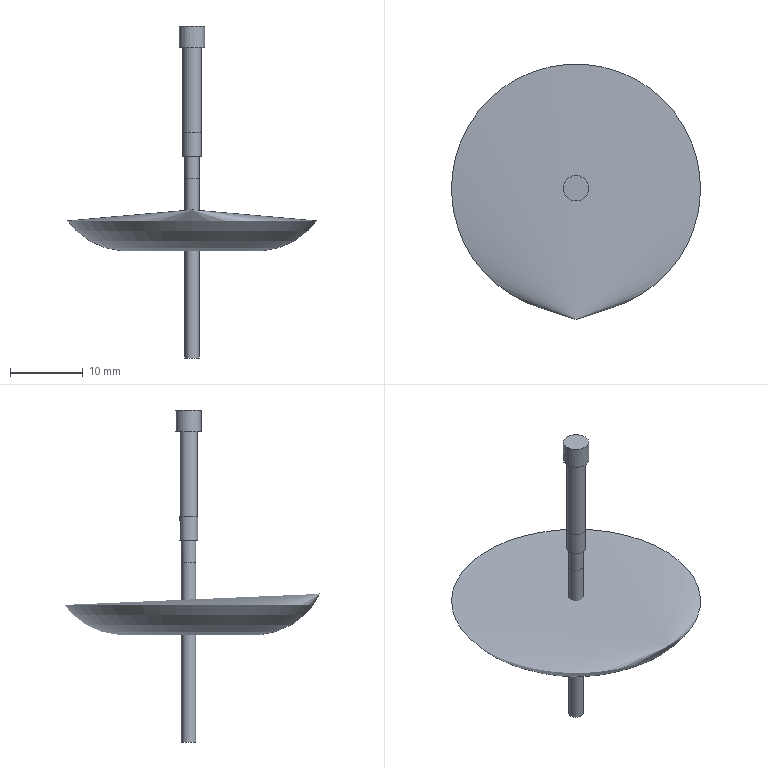Part | NX | features BREP 2 | 2 solids | 14 faces | cylinder 6 | plane 6 | torus 2 | commonest cylinder face diameters 2 x2 2.5 x2 3.5 x2
STEP:
#1=CARTESIAN_POINT('',(1.75,0.,17.));
#2=VERTEX_POINT('',#1);
#3=CARTESIAN_POINT('',(0.,0.,17.));
#4=DIRECTION('',(0.,0.,1.));
#5=DIRECTION('',(1.,0.,0.));
#6=AXIS2_PLACEMENT_3D('',#3,#4,#5);
#7=CIRCLE('',#6,1.75);
#8=EDGE_CURVE('',#2,#2,#7,.T.);
#9=ORIENTED_EDGE('',*,*,#8,.T.);
#10=EDGE_LOOP('',(#9));
#11=FACE_BOUND('',#10,.T.);
#12=CARTESIAN_POINT('',(1.75,0.,20.));
#13=VERTEX_POINT('',#12);
#14=CARTESIAN_POINT('',(0.,0.,20.));
#15=DIRECTION('',(0.,0.,1.));
#16=DIRECTION('',(1.,0.,0.));
#17=AXIS2_PLACEMENT_3D('',#14,#15,#16);
#18=CIRCLE('',#17,1.75);
#19=EDGE_CURVE('',#13,#13,#18,.T.);
#20=ORIENTED_EDGE('',*,*,#19,.F.);
#21=EDGE_LOOP('',(#20));
#22=FACE_BOUND('',#21,.T.);
#23=CARTESIAN_POINT('',(0.,0.,17.));
#24=DIRECTION('',(0.,0.,1.));
#25=DIRECTION('',(-1.,0.,0.));
#26=AXIS2_PLACEMENT_3D('',#23,#24,#25);
#27=CYLINDRICAL_SURFACE('',#26,1.75);
#28=ADVANCED_FACE('',(#11,#22),#27,.T.);
#29=CARTESIAN_POINT('',(-1.25,0.,17.));
#30=VERTEX_POINT('',#29);
#31=CARTESIAN_POINT('',(0.,0.,17.));
#32=DIRECTION('',(0.,0.,-1.));
#33=DIRECTION('',(-1.,0.,0.));
#34=AXIS2_PLACEMENT_3D('',#31,#32,#33);
#35=CIRCLE('',#34,1.25);
#36=EDGE_CURVE('',#30,#30,#35,.T.);
#37=ORIENTED_EDGE('',*,*,#36,.F.);
#38=EDGE_LOOP('',(#37));
#39=FACE_BOUND('',#38,.T.);
#40=ORIENTED_EDGE('',*,*,#8,.F.);
#41=EDGE_LOOP('',(#40));
#42=FACE_BOUND('',#41,.T.);
#43=CARTESIAN_POINT('',(0.,0.,17.));
#44=DIRECTION('',(0.,0.,1.));
#45=DIRECTION('',(-1.,0.,0.));
#46=AXIS2_PLACEMENT_3D('',#43,#44,#45);
#47=PLANE('',#46);
#48=ADVANCED_FACE('',(#39,#42),#47,.F.);
#49=ORIENTED_EDGE('',*,*,#19,.T.);
#50=EDGE_LOOP('',(#49));
#51=FACE_BOUND('',#50,.T.);
#52=CARTESIAN_POINT('',(0.,0.,20.));
#53=DIRECTION('',(0.,0.,1.));
#54=DIRECTION('',(-1.,0.,0.));
#55=AXIS2_PLACEMENT_3D('',#52,#53,#54);
#56=PLANE('',#55);
#57=ADVANCED_FACE('',(#51),#56,.T.);
#58=CARTESIAN_POINT('',(-1.25,0.,5.322));
#59=VERTEX_POINT('',#58);
#60=CARTESIAN_POINT('',(0.,0.,5.322));
#61=DIRECTION('',(0.,0.,-1.));
#62=DIRECTION('',(-1.,0.,0.));
#63=AXIS2_PLACEMENT_3D('',#60,#61,#62);
#64=CIRCLE('',#63,1.25);
#65=EDGE_CURVE('',#59,#59,#64,.T.);
#66=ORIENTED_EDGE('',*,*,#65,.F.);
#67=EDGE_LOOP('',(#66));
#68=FACE_BOUND('',#67,.T.);
#69=ORIENTED_EDGE('',*,*,#36,.T.);
#70=EDGE_LOOP('',(#69));
#71=FACE_BOUND('',#70,.T.);
#72=CARTESIAN_POINT('',(0.,0.,17.));
#73=DIRECTION('',(0.,0.,-1.));
#74=DIRECTION('',(1.,0.,0.));
#75=AXIS2_PLACEMENT_3D('',#72,#73,#74);
#76=CYLINDRICAL_SURFACE('',#75,1.25);
#77=ADVANCED_FACE('',(#68,#71),#76,.T.);
#78=CARTESIAN_POINT('',(1.,0.,3.1));
#79=VERTEX_POINT('',#78);
#80=CARTESIAN_POINT('',(0.,0.,3.1));
#81=DIRECTION('',(0.,0.,-1.));
#82=DIRECTION('',(1.,0.,0.));
#83=AXIS2_PLACEMENT_3D('',#80,#81,#82);
#84=CIRCLE('',#83,1.);
#85=EDGE_CURVE('',#79,#79,#84,.T.);
#86=ORIENTED_EDGE('',*,*,#85,.T.);
#87=EDGE_LOOP('',(#86));
#88=FACE_BOUND('',#87,.T.);
#89=CARTESIAN_POINT('',(-1.,0.,-0.9));
#90=VERTEX_POINT('',#89);
#91=CARTESIAN_POINT('',(0.,0.,-0.9));
#92=DIRECTION('',(0.,0.,-1.));
#93=DIRECTION('',(-1.,0.,0.));
#94=AXIS2_PLACEMENT_3D('',#91,#92,#93);
#95=CIRCLE('',#94,1.);
#96=EDGE_CURVE('',#90,#90,#95,.T.);
#97=ORIENTED_EDGE('',*,*,#96,.F.);
#98=EDGE_LOOP('',(#97));
#99=FACE_BOUND('',#98,.T.);
#100=CARTESIAN_POINT('',(0.,0.,5.322));
#101=DIRECTION('',(0.,0.,-1.));
#102=DIRECTION('',(1.,0.,0.));
#103=AXIS2_PLACEMENT_3D('',#100,#101,#102);
#104=CYLINDRICAL_SURFACE('',#103,1.);
#105=ADVANCED_FACE('',(#88,#99),#104,.T.);
#106=ORIENTED_EDGE('',*,*,#65,.T.);
#107=EDGE_LOOP('',(#106));
#108=FACE_BOUND('',#107,.T.);
#109=ORIENTED_EDGE('',*,*,#85,.F.);
#110=EDGE_LOOP('',(#109));
#111=FACE_BOUND('',#110,.T.);
#112=CARTESIAN_POINT('',(0.,0.,3.1));
#113=DIRECTION('',(0.,0.,1.));
#114=DIRECTION('',(-1.,0.,0.));
#115=AXIS2_PLACEMENT_3D('',#112,#113,#114);
#116=TOROIDAL_SURFACE('',#115,11.,10.);
#117=ADVANCED_FACE('',(#108,#111),#116,.F.);
#118=ORIENTED_EDGE('',*,*,#96,.T.);
#119=EDGE_LOOP('',(#118));
#120=FACE_BOUND('',#119,.T.);
#121=CARTESIAN_POINT('',(0.,0.,-5.259));
#122=VERTEX_POINT('',#121);
#123=VERTEX_LOOP('',#122);
#124=FACE_BOUND('',#123,.T.);
#125=CARTESIAN_POINT('',(0.,0.,-0.9));
#126=DIRECTION('',(0.,0.,1.));
#127=DIRECTION('',(0.,-1.,0.));
#128=AXIS2_PLACEMENT_3D('',#125,#126,#127);
#129=DEGENERATE_TOROIDAL_SURFACE('',#128,9.,10.,.F.);
#130=ADVANCED_FACE('',(#120,#124),#129,.F.);
#131=CLOSED_SHELL('',(#28,#48,#57,#77,#105,#117,#130));
#132=MANIFOLD_SOLID_BREP('',#131);
#133=CARTESIAN_POINT('',(1.75,0.,17.));
#134=VERTEX_POINT('',#133);
#135=CARTESIAN_POINT('',(0.,0.,17.));
#136=DIRECTION('',(0.,0.,1.));
#137=DIRECTION('',(1.,0.,0.));
#138=AXIS2_PLACEMENT_3D('',#135,#136,#137);
#139=CIRCLE('',#138,1.75);
#140=EDGE_CURVE('',#134,#134,#139,.T.);
#141=ORIENTED_EDGE('',*,*,#140,.T.);
#142=EDGE_LOOP('',(#141));
#143=FACE_BOUND('',#142,.T.);
#144=CARTESIAN_POINT('',(1.75,0.,20.));
#145=VERTEX_POINT('',#144);
#146=CARTESIAN_POINT('',(0.,0.,20.));
#147=DIRECTION('',(0.,0.,1.));
#148=DIRECTION('',(1.,0.,0.));
#149=AXIS2_PLACEMENT_3D('',#146,#147,#148);
#150=CIRCLE('',#149,1.75);
#151=EDGE_CURVE('',#145,#145,#150,.T.);
#152=ORIENTED_EDGE('',*,*,#151,.F.);
#153=EDGE_LOOP('',(#152));
#154=FACE_BOUND('',#153,.T.);
#155=CARTESIAN_POINT('',(0.,0.,17.));
#156=DIRECTION('',(0.,0.,1.));
#157=DIRECTION('',(-1.,0.,0.));
#158=AXIS2_PLACEMENT_3D('',#155,#156,#157);
#159=CYLINDRICAL_SURFACE('',#158,1.75);
#160=ADVANCED_FACE('',(#143,#154),#159,.T.);
#161=CARTESIAN_POINT('',(-1.25,0.,17.));
#162=VERTEX_POINT('',#161);
#163=CARTESIAN_POINT('',(0.,0.,17.));
#164=DIRECTION('',(0.,0.,-1.));
#165=DIRECTION('',(-1.,0.,0.));
#166=AXIS2_PLACEMENT_3D('',#163,#164,#165);
#167=CIRCLE('',#166,1.25);
#168=EDGE_CURVE('',#162,#162,#167,.T.);
#169=ORIENTED_EDGE('',*,*,#168,.F.);
#170=EDGE_LOOP('',(#169));
#171=FACE_BOUND('',#170,.T.);
#172=ORIENTED_EDGE('',*,*,#140,.F.);
#173=EDGE_LOOP('',(#172));
#174=FACE_BOUND('',#173,.T.);
#175=CARTESIAN_POINT('',(0.,0.,17.));
#176=DIRECTION('',(0.,0.,1.));
#177=DIRECTION('',(-1.,0.,0.));
#178=AXIS2_PLACEMENT_3D('',#175,#176,#177);
#179=PLANE('',#178);
#180=ADVANCED_FACE('',(#171,#174),#179,.F.);
#181=ORIENTED_EDGE('',*,*,#151,.T.);
#182=EDGE_LOOP('',(#181));
#183=FACE_BOUND('',#182,.T.);
#184=CARTESIAN_POINT('',(0.,0.,20.));
#185=DIRECTION('',(0.,0.,1.));
#186=DIRECTION('',(-1.,0.,0.));
#187=AXIS2_PLACEMENT_3D('',#184,#185,#186);
#188=PLANE('',#187);
#189=ADVANCED_FACE('',(#183),#188,.T.);
#190=CARTESIAN_POINT('',(1.25,0.,2.1));
#191=VERTEX_POINT('',#190);
#192=CARTESIAN_POINT('',(0.,0.,2.1));
#193=DIRECTION('',(0.,0.,-1.));
#194=DIRECTION('',(1.,0.,0.));
#195=AXIS2_PLACEMENT_3D('',#192,#193,#194);
#196=CIRCLE('',#195,1.25);
#197=EDGE_CURVE('',#191,#191,#196,.T.);
#198=ORIENTED_EDGE('',*,*,#197,.F.);
#199=EDGE_LOOP('',(#198));
#200=FACE_BOUND('',#199,.T.);
#201=ORIENTED_EDGE('',*,*,#168,.T.);
#202=EDGE_LOOP('',(#201));
#203=FACE_BOUND('',#202,.T.);
#204=CARTESIAN_POINT('',(0.,0.,17.));
#205=DIRECTION('',(0.,0.,-1.));
#206=DIRECTION('',(1.,0.,0.));
#207=AXIS2_PLACEMENT_3D('',#204,#205,#206);
#208=CYLINDRICAL_SURFACE('',#207,1.25);
#209=ADVANCED_FACE('',(#200,#203),#208,.T.);
#210=CARTESIAN_POINT('',(1.,0.,2.1));
#211=VERTEX_POINT('',#210);
#212=CARTESIAN_POINT('',(0.,0.,2.1));
#213=DIRECTION('',(0.,0.,1.));
#214=DIRECTION('',(1.,0.,0.));
#215=AXIS2_PLACEMENT_3D('',#212,#213,#214);
#216=CIRCLE('',#215,1.);
#217=EDGE_CURVE('',#211,#211,#216,.T.);
#218=ORIENTED_EDGE('',*,*,#217,.T.);
#219=EDGE_LOOP('',(#218));
#220=FACE_BOUND('',#219,.T.);
#221=ORIENTED_EDGE('',*,*,#197,.T.);
#222=EDGE_LOOP('',(#221));
#223=FACE_BOUND('',#222,.T.);
#224=CARTESIAN_POINT('',(0.,0.,2.1));
#225=DIRECTION('',(0.,0.,1.));
#226=DIRECTION('',(-1.,0.,0.));
#227=AXIS2_PLACEMENT_3D('',#224,#225,#226);
#228=PLANE('',#227);
#229=ADVANCED_FACE('',(#220,#223),#228,.F.);
#230=CARTESIAN_POINT('',(1.,0.,-25.6));
#231=VERTEX_POINT('',#230);
#232=CARTESIAN_POINT('',(0.,0.,-25.6));
#233=DIRECTION('',(0.,0.,1.));
#234=DIRECTION('',(1.,0.,0.));
#235=AXIS2_PLACEMENT_3D('',#232,#233,#234);
#236=CIRCLE('',#235,1.);
#237=EDGE_CURVE('',#231,#231,#236,.T.);
#238=ORIENTED_EDGE('',*,*,#237,.T.);
#239=EDGE_LOOP('',(#238));
#240=FACE_BOUND('',#239,.T.);
#241=ORIENTED_EDGE('',*,*,#217,.F.);
#242=EDGE_LOOP('',(#241));
#243=FACE_BOUND('',#242,.T.);
#244=CARTESIAN_POINT('',(0.,0.,-25.6));
#245=DIRECTION('',(0.,0.,1.));
#246=DIRECTION('',(-1.,0.,0.));
#247=AXIS2_PLACEMENT_3D('',#244,#245,#246);
#248=CYLINDRICAL_SURFACE('',#247,1.);
#249=ADVANCED_FACE('',(#240,#243),#248,.T.);
#250=ORIENTED_EDGE('',*,*,#237,.F.);
#251=EDGE_LOOP('',(#250));
#252=FACE_BOUND('',#251,.T.);
#253=CARTESIAN_POINT('',(0.,0.,-25.6));
#254=DIRECTION('',(0.,0.,1.));
#255=DIRECTION('',(-1.,0.,0.));
#256=AXIS2_PLACEMENT_3D('',#253,#254,#255);
#257=PLANE('',#256);
#258=ADVANCED_FACE('',(#252),#257,.F.);
#259=CLOSED_SHELL('',(#160,#180,#189,#209,#229,#249,#258));
#260=MANIFOLD_SOLID_BREP('',#259);
#261=(LENGTH_UNIT()NAMED_UNIT(*)SI_UNIT(.MILLI.,.METRE.));
#262=UNCERTAINTY_MEASURE_WITH_UNIT(LENGTH_MEASURE(0.00001),#261,'','');
#263=(NAMED_UNIT(*)PLANE_ANGLE_UNIT()SI_UNIT($,.RADIAN.));
#264=(NAMED_UNIT(*)SI_UNIT($,.STERADIAN.)SOLID_ANGLE_UNIT());
#265=(GEOMETRIC_REPRESENTATION_CONTEXT(3)GLOBAL_UNCERTAINTY_ASSIGNED_CONTEXT((#262))GLOBAL_UNIT_ASSIGNED_CONTEXT((#261,#263,#264))REPRESENTATION_CONTEXT('',''));
#266=ADVANCED_BREP_SHAPE_REPRESENTATION('',(#132,#260),#265);